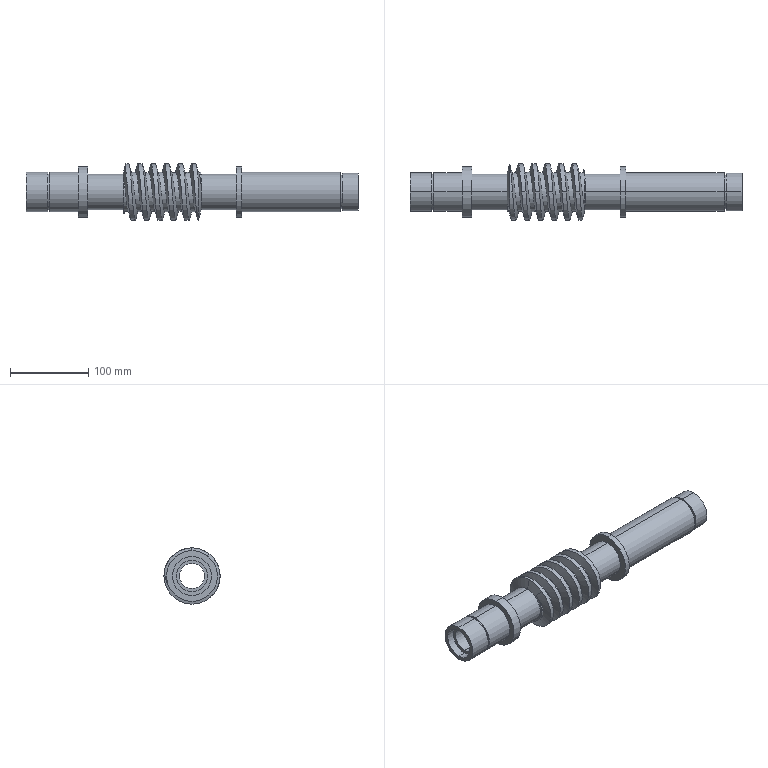Part | SolidWorks | features ICE 13, Chamfer 1, Cut 1, Extrusion 1, Helix 1, RevCut 1, SweepCut 1 | 1 solid | 63 faces | box 425 x 72 x 72 mm | volume 557558 mm3 | cylinder 41 | plane 13 | cone 6 | spline 3 | commonest cylinder face diameters 72 x13 50 x6 46 x4 65 x4 32 x2 33 x2